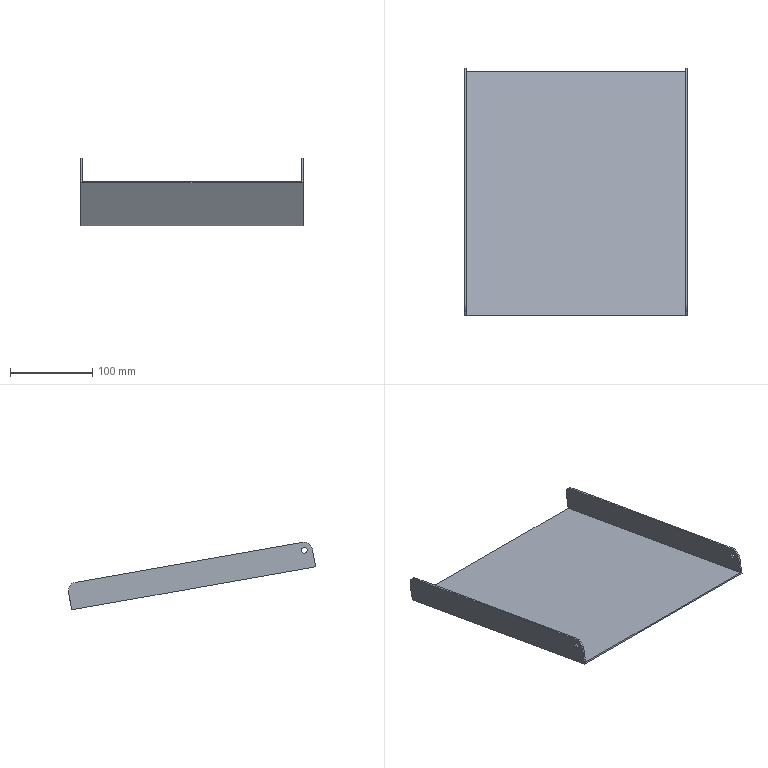Part | NX | features HB 2 | 1 solid | 16 faces | box 270 x 300.028 x 82.132 mm | volume 198086 mm3 | plane 10 | cylinder 6 | commonest cylinder face diameters 20 x4 7 x2
STEP:
#1=CARTESIAN_POINT('',(296.,686.06,-368.904));
#2=VERTEX_POINT('',#1);
#3=CARTESIAN_POINT('',(296.,686.966,-372.285));
#4=DIRECTION('',(1.,0.,0.));
#5=DIRECTION('',(0.,-0.2588,0.9659));
#6=AXIS2_PLACEMENT_3D('',#3,#4,#5);
#7=CIRCLE('',#6,3.5);
#8=EDGE_CURVE('',#2,#2,#7,.T.);
#9=ORIENTED_EDGE('',*,*,#8,.T.);
#10=EDGE_LOOP('',(#9));
#11=FACE_BOUND('',#10,.T.);
#12=CARTESIAN_POINT('',(294.,686.06,-368.904));
#13=VERTEX_POINT('',#12);
#14=CARTESIAN_POINT('',(294.,686.966,-372.285));
#15=DIRECTION('',(-1.,0.,0.));
#16=DIRECTION('',(0.,-0.2588,0.9659));
#17=AXIS2_PLACEMENT_3D('',#14,#15,#16);
#18=CIRCLE('',#17,3.5);
#19=EDGE_CURVE('',#13,#13,#18,.T.);
#20=ORIENTED_EDGE('',*,*,#19,.T.);
#21=EDGE_LOOP('',(#20));
#22=FACE_BOUND('',#21,.T.);
#23=CARTESIAN_POINT('',(-406.,686.966,-372.285));
#24=DIRECTION('',(1.,0.,0.));
#25=DIRECTION('',(0.,0.2588,-0.9659));
#26=AXIS2_PLACEMENT_3D('',#23,#24,#25);
#27=CYLINDRICAL_SURFACE('',#26,3.5);
#28=ADVANCED_FACE('',(#11,#22),#27,.F.);
#29=CARTESIAN_POINT('',(296.,965.062,-411.167));
#30=VERTEX_POINT('',#29);
#31=CARTESIAN_POINT('',(296.,688.702,-362.437));
#32=VERTEX_POINT('',#31);
#33=CARTESIAN_POINT('',(296.,564.245,-340.492));
#34=DIRECTION('',(0.,-0.9848,0.1736));
#35=VECTOR('',#34,1000.);
#36=LINE('',#33,#35);
#37=EDGE_CURVE('',#30,#32,#36,.T.);
#38=ORIENTED_EDGE('',*,*,#37,.F.);
#39=CARTESIAN_POINT('',(294.,965.062,-411.167));
#40=VERTEX_POINT('',#39);
#41=CARTESIAN_POINT('',(200.,965.062,-411.167));
#42=DIRECTION('',(1.,0.,0.));
#43=VECTOR('',#42,1000.);
#44=LINE('',#41,#43);
#45=EDGE_CURVE('',#40,#30,#44,.T.);
#46=ORIENTED_EDGE('',*,*,#45,.F.);
#47=CARTESIAN_POINT('',(294.,688.702,-362.437));
#48=VERTEX_POINT('',#47);
#49=CARTESIAN_POINT('',(294.,564.245,-340.492));
#50=DIRECTION('',(0.,-0.9848,0.1736));
#51=VECTOR('',#50,1000.);
#52=LINE('',#49,#51);
#53=EDGE_CURVE('',#40,#48,#52,.T.);
#54=ORIENTED_EDGE('',*,*,#53,.T.);
#55=CARTESIAN_POINT('',(200.,688.702,-362.437));
#56=DIRECTION('',(1.,0.,0.));
#57=VECTOR('',#56,1000.);
#58=LINE('',#55,#57);
#59=EDGE_CURVE('',#48,#32,#58,.T.);
#60=ORIENTED_EDGE('',*,*,#59,.T.);
#61=EDGE_LOOP('',(#38,#46,#54,#60));
#62=FACE_BOUND('',#61,.T.);
#63=CARTESIAN_POINT('',(200.,564.245,-340.492));
#64=DIRECTION('',(0.,-0.1736,-0.9848));
#65=DIRECTION('',(0.,0.9848,-0.1736));
#66=AXIS2_PLACEMENT_3D('',#63,#64,#65);
#67=PLANE('',#66);
#68=ADVANCED_FACE('',(#62),#67,.F.);
#69=CARTESIAN_POINT('',(296.,973.174,-422.751));
#70=VERTEX_POINT('',#69);
#71=CARTESIAN_POINT('',(296.,963.326,-421.015));
#72=DIRECTION('',(-1.,0.,0.));
#73=DIRECTION('',(0.,-0.2588,0.9659));
#74=AXIS2_PLACEMENT_3D('',#71,#72,#73);
#75=CIRCLE('',#74,10.);
#76=EDGE_CURVE('',#30,#70,#75,.T.);
#77=ORIENTED_EDGE('',*,*,#76,.T.);
#78=CARTESIAN_POINT('',(294.,973.174,-422.751));
#79=VERTEX_POINT('',#78);
#80=CARTESIAN_POINT('',(200.,973.174,-422.751));
#81=DIRECTION('',(-1.,0.,0.));
#82=VECTOR('',#81,1000.);
#83=LINE('',#80,#82);
#84=EDGE_CURVE('',#70,#79,#83,.T.);
#85=ORIENTED_EDGE('',*,*,#84,.T.);
#86=CARTESIAN_POINT('',(294.,963.326,-421.015));
#87=DIRECTION('',(1.,0.,0.));
#88=DIRECTION('',(0.,-0.2588,0.9659));
#89=AXIS2_PLACEMENT_3D('',#86,#87,#88);
#90=CIRCLE('',#89,10.);
#91=EDGE_CURVE('',#79,#40,#90,.T.);
#92=ORIENTED_EDGE('',*,*,#91,.T.);
#93=ORIENTED_EDGE('',*,*,#45,.T.);
#94=EDGE_LOOP('',(#77,#85,#92,#93));
#95=FACE_BOUND('',#94,.T.);
#96=CARTESIAN_POINT('',(200.,963.326,-421.015));
#97=DIRECTION('',(-1.,0.,0.));
#98=DIRECTION('',(0.,-0.2588,0.9659));
#99=AXIS2_PLACEMENT_3D('',#96,#97,#98);
#100=CYLINDRICAL_SURFACE('',#99,10.);
#101=ADVANCED_FACE('',(#95),#100,.T.);
#102=ORIENTED_EDGE('',*,*,#53,.F.);
#103=ORIENTED_EDGE('',*,*,#91,.F.);
#104=CARTESIAN_POINT('',(294.,969.354,-444.417));
#105=VERTEX_POINT('',#104);
#106=CARTESIAN_POINT('',(294.,969.701,-442.448));
#107=DIRECTION('',(0.,0.1736,0.9848));
#108=VECTOR('',#107,1000.);
#109=LINE('',#106,#108);
#110=EDGE_CURVE('',#105,#79,#109,.T.);
#111=ORIENTED_EDGE('',*,*,#110,.F.);
#112=CARTESIAN_POINT('',(294.,673.298,-392.215));
#113=VERTEX_POINT('',#112);
#114=CARTESIAN_POINT('',(294.,558.689,-372.006));
#115=DIRECTION('',(0.,0.9848,-0.1736));
#116=VECTOR('',#115,1000.);
#117=LINE('',#114,#116);
#118=EDGE_CURVE('',#113,#105,#117,.T.);
#119=ORIENTED_EDGE('',*,*,#118,.F.);
#120=CARTESIAN_POINT('',(294.,677.118,-370.549));
#121=VERTEX_POINT('',#120);
#122=CARTESIAN_POINT('',(294.,673.645,-390.245));
#123=DIRECTION('',(0.,0.1736,0.9848));
#124=VECTOR('',#123,1000.);
#125=LINE('',#122,#124);
#126=EDGE_CURVE('',#113,#121,#125,.T.);
#127=ORIENTED_EDGE('',*,*,#126,.T.);
#128=CARTESIAN_POINT('',(294.,686.966,-372.285));
#129=DIRECTION('',(-1.,0.,0.));
#130=DIRECTION('',(0.,0.5736,0.8192));
#131=AXIS2_PLACEMENT_3D('',#128,#129,#130);
#132=CIRCLE('',#131,10.);
#133=EDGE_CURVE('',#121,#48,#132,.T.);
#134=ORIENTED_EDGE('',*,*,#133,.T.);
#135=EDGE_LOOP('',(#102,#103,#111,#119,#127,#134));
#136=FACE_BOUND('',#135,.T.);
#137=ORIENTED_EDGE('',*,*,#19,.F.);
#138=EDGE_LOOP('',(#137));
#139=FACE_BOUND('',#138,.T.);
#140=CARTESIAN_POINT('',(294.,559.036,-370.036));
#141=DIRECTION('',(1.,0.,0.));
#142=DIRECTION('',(0.,0.2588,-0.9659));
#143=AXIS2_PLACEMENT_3D('',#140,#141,#142);
#144=PLANE('',#143);
#145=ADVANCED_FACE('',(#136,#139),#144,.F.);
#146=CARTESIAN_POINT('',(296.,677.118,-370.549));
#147=VERTEX_POINT('',#146);
#148=CARTESIAN_POINT('',(296.,686.966,-372.285));
#149=DIRECTION('',(1.,0.,0.));
#150=DIRECTION('',(0.,0.5736,0.8192));
#151=AXIS2_PLACEMENT_3D('',#148,#149,#150);
#152=CIRCLE('',#151,10.);
#153=EDGE_CURVE('',#32,#147,#152,.T.);
#154=ORIENTED_EDGE('',*,*,#153,.F.);
#155=ORIENTED_EDGE('',*,*,#59,.F.);
#156=ORIENTED_EDGE('',*,*,#133,.F.);
#157=CARTESIAN_POINT('',(260.,677.118,-370.549));
#158=DIRECTION('',(-1.,0.,0.));
#159=VECTOR('',#158,1000.);
#160=LINE('',#157,#159);
#161=EDGE_CURVE('',#147,#121,#160,.T.);
#162=ORIENTED_EDGE('',*,*,#161,.F.);
#163=EDGE_LOOP('',(#154,#155,#156,#162));
#164=FACE_BOUND('',#163,.T.);
#165=CARTESIAN_POINT('',(200.,686.966,-372.285));
#166=DIRECTION('',(-1.,0.,0.));
#167=DIRECTION('',(0.,0.5736,0.8192));
#168=AXIS2_PLACEMENT_3D('',#165,#166,#167);
#169=CYLINDRICAL_SURFACE('',#168,10.);
#170=ADVANCED_FACE('',(#164),#169,.T.);
#171=ORIENTED_EDGE('',*,*,#76,.F.);
#172=ORIENTED_EDGE('',*,*,#37,.T.);
#173=ORIENTED_EDGE('',*,*,#153,.T.);
#174=CARTESIAN_POINT('',(296.,673.645,-390.245));
#175=VERTEX_POINT('',#174);
#176=CARTESIAN_POINT('',(296.,673.645,-390.245));
#177=DIRECTION('',(0.,0.1736,0.9848));
#178=VECTOR('',#177,1000.);
#179=LINE('',#176,#178);
#180=EDGE_CURVE('',#175,#147,#179,.T.);
#181=ORIENTED_EDGE('',*,*,#180,.F.);
#182=CARTESIAN_POINT('',(296.,969.701,-442.448));
#183=VERTEX_POINT('',#182);
#184=CARTESIAN_POINT('',(296.,559.036,-370.036));
#185=DIRECTION('',(0.,-0.9848,0.1736));
#186=VECTOR('',#185,1000.);
#187=LINE('',#184,#186);
#188=EDGE_CURVE('',#183,#175,#187,.T.);
#189=ORIENTED_EDGE('',*,*,#188,.F.);
#190=CARTESIAN_POINT('',(296.,969.701,-442.448));
#191=DIRECTION('',(0.,0.1736,0.9848));
#192=VECTOR('',#191,1000.);
#193=LINE('',#190,#192);
#194=EDGE_CURVE('',#183,#70,#193,.T.);
#195=ORIENTED_EDGE('',*,*,#194,.T.);
#196=EDGE_LOOP('',(#171,#172,#173,#181,#189,#195));
#197=FACE_BOUND('',#196,.T.);
#198=ORIENTED_EDGE('',*,*,#8,.F.);
#199=EDGE_LOOP('',(#198));
#200=FACE_BOUND('',#199,.T.);
#201=CARTESIAN_POINT('',(296.,559.036,-370.036));
#202=DIRECTION('',(1.,0.,0.));
#203=DIRECTION('',(0.,-0.2588,0.9659));
#204=AXIS2_PLACEMENT_3D('',#201,#202,#203);
#205=PLANE('',#204);
#206=ADVANCED_FACE('',(#197,#200),#205,.T.);
#207=CARTESIAN_POINT('',(562.,673.645,-390.245));
#208=VERTEX_POINT('',#207);
#209=CARTESIAN_POINT('',(260.,673.645,-390.245));
#210=DIRECTION('',(1.,0.,0.));
#211=VECTOR('',#210,1000.);
#212=LINE('',#209,#211);
#213=EDGE_CURVE('',#175,#208,#212,.T.);
#214=ORIENTED_EDGE('',*,*,#213,.F.);
#215=ORIENTED_EDGE('',*,*,#180,.T.);
#216=ORIENTED_EDGE('',*,*,#161,.T.);
#217=ORIENTED_EDGE('',*,*,#126,.F.);
#218=CARTESIAN_POINT('',(564.,673.298,-392.215));
#219=VERTEX_POINT('',#218);
#220=CARTESIAN_POINT('',(260.,673.298,-392.215));
#221=DIRECTION('',(1.,0.,0.));
#222=VECTOR('',#221,1000.);
#223=LINE('',#220,#222);
#224=EDGE_CURVE('',#113,#219,#223,.T.);
#225=ORIENTED_EDGE('',*,*,#224,.T.);
#226=CARTESIAN_POINT('',(564.,677.118,-370.549));
#227=VERTEX_POINT('',#226);
#228=CARTESIAN_POINT('',(564.,673.645,-390.245));
#229=DIRECTION('',(0.,0.1736,0.9848));
#230=VECTOR('',#229,1000.);
#231=LINE('',#228,#230);
#232=EDGE_CURVE('',#219,#227,#231,.T.);
#233=ORIENTED_EDGE('',*,*,#232,.T.);
#234=CARTESIAN_POINT('',(562.,677.118,-370.549));
#235=VERTEX_POINT('',#234);
#236=CARTESIAN_POINT('',(260.,677.118,-370.549));
#237=DIRECTION('',(-1.,0.,0.));
#238=VECTOR('',#237,1000.);
#239=LINE('',#236,#238);
#240=EDGE_CURVE('',#227,#235,#239,.T.);
#241=ORIENTED_EDGE('',*,*,#240,.T.);
#242=CARTESIAN_POINT('',(562.,673.645,-390.245));
#243=DIRECTION('',(0.,0.1736,0.9848));
#244=VECTOR('',#243,1000.);
#245=LINE('',#242,#244);
#246=EDGE_CURVE('',#208,#235,#245,.T.);
#247=ORIENTED_EDGE('',*,*,#246,.F.);
#248=EDGE_LOOP('',(#214,#215,#216,#217,#225,#233,#241,#247));
#249=FACE_BOUND('',#248,.T.);
#250=CARTESIAN_POINT('',(260.,673.645,-390.245));
#251=DIRECTION('',(0.,0.9848,-0.1736));
#252=DIRECTION('',(0.,-0.1736,-0.9848));
#253=AXIS2_PLACEMENT_3D('',#250,#251,#252);
#254=PLANE('',#253);
#255=ADVANCED_FACE('',(#249),#254,.F.);
#256=ORIENTED_EDGE('',*,*,#194,.F.);
#257=CARTESIAN_POINT('',(562.,969.701,-442.448));
#258=VERTEX_POINT('',#257);
#259=CARTESIAN_POINT('',(260.,969.701,-442.448));
#260=DIRECTION('',(1.,0.,0.));
#261=VECTOR('',#260,1000.);
#262=LINE('',#259,#261);
#263=EDGE_CURVE('',#183,#258,#262,.T.);
#264=ORIENTED_EDGE('',*,*,#263,.T.);
#265=CARTESIAN_POINT('',(562.,973.174,-422.751));
#266=VERTEX_POINT('',#265);
#267=CARTESIAN_POINT('',(562.,969.701,-442.448));
#268=DIRECTION('',(0.,0.1736,0.9848));
#269=VECTOR('',#268,1000.);
#270=LINE('',#267,#269);
#271=EDGE_CURVE('',#258,#266,#270,.T.);
#272=ORIENTED_EDGE('',*,*,#271,.T.);
#273=CARTESIAN_POINT('',(564.,973.174,-422.751));
#274=VERTEX_POINT('',#273);
#275=CARTESIAN_POINT('',(259.,973.174,-422.751));
#276=DIRECTION('',(-1.,0.,0.));
#277=VECTOR('',#276,1000.);
#278=LINE('',#275,#277);
#279=EDGE_CURVE('',#274,#266,#278,.T.);
#280=ORIENTED_EDGE('',*,*,#279,.F.);
#281=CARTESIAN_POINT('',(564.,969.354,-444.417));
#282=VERTEX_POINT('',#281);
#283=CARTESIAN_POINT('',(564.,969.701,-442.448));
#284=DIRECTION('',(0.,0.1736,0.9848));
#285=VECTOR('',#284,1000.);
#286=LINE('',#283,#285);
#287=EDGE_CURVE('',#282,#274,#286,.T.);
#288=ORIENTED_EDGE('',*,*,#287,.F.);
#289=CARTESIAN_POINT('',(260.,969.354,-444.417));
#290=DIRECTION('',(1.,0.,0.));
#291=VECTOR('',#290,1000.);
#292=LINE('',#289,#291);
#293=EDGE_CURVE('',#105,#282,#292,.T.);
#294=ORIENTED_EDGE('',*,*,#293,.F.);
#295=ORIENTED_EDGE('',*,*,#110,.T.);
#296=ORIENTED_EDGE('',*,*,#84,.F.);
#297=EDGE_LOOP('',(#256,#264,#272,#280,#288,#294,#295,#296));
#298=FACE_BOUND('',#297,.T.);
#299=CARTESIAN_POINT('',(260.,969.701,-442.448));
#300=DIRECTION('',(0.,-0.9848,0.1736));
#301=DIRECTION('',(0.,-0.1736,-0.9848));
#302=AXIS2_PLACEMENT_3D('',#299,#300,#301);
#303=PLANE('',#302);
#304=ADVANCED_FACE('',(#298),#303,.F.);
#305=ORIENTED_EDGE('',*,*,#118,.T.);
#306=ORIENTED_EDGE('',*,*,#293,.T.);
#307=CARTESIAN_POINT('',(564.,558.689,-372.006));
#308=DIRECTION('',(0.,-0.9848,0.1736));
#309=VECTOR('',#308,1000.);
#310=LINE('',#307,#309);
#311=EDGE_CURVE('',#282,#219,#310,.T.);
#312=ORIENTED_EDGE('',*,*,#311,.T.);
#313=ORIENTED_EDGE('',*,*,#224,.F.);
#314=EDGE_LOOP('',(#305,#306,#312,#313));
#315=FACE_BOUND('',#314,.T.);
#316=CARTESIAN_POINT('',(260.,558.689,-372.006));
#317=DIRECTION('',(0.,0.1736,0.9848));
#318=DIRECTION('',(1.,0.,0.));
#319=AXIS2_PLACEMENT_3D('',#316,#317,#318);
#320=PLANE('',#319);
#321=ADVANCED_FACE('',(#315),#320,.F.);
#322=ORIENTED_EDGE('',*,*,#263,.F.);
#323=ORIENTED_EDGE('',*,*,#188,.T.);
#324=ORIENTED_EDGE('',*,*,#213,.T.);
#325=CARTESIAN_POINT('',(562.,559.036,-370.036));
#326=DIRECTION('',(0.,0.9848,-0.1736));
#327=VECTOR('',#326,1000.);
#328=LINE('',#325,#327);
#329=EDGE_CURVE('',#208,#258,#328,.T.);
#330=ORIENTED_EDGE('',*,*,#329,.T.);
#331=EDGE_LOOP('',(#322,#323,#324,#330));
#332=FACE_BOUND('',#331,.T.);
#333=CARTESIAN_POINT('',(260.,559.036,-370.036));
#334=DIRECTION('',(0.,0.1736,0.9848));
#335=DIRECTION('',(1.,0.,0.));
#336=AXIS2_PLACEMENT_3D('',#333,#334,#335);
#337=PLANE('',#336);
#338=ADVANCED_FACE('',(#332),#337,.T.);
#339=CARTESIAN_POINT('',(564.,687.872,-375.666));
#340=VERTEX_POINT('',#339);
#341=CARTESIAN_POINT('',(564.,686.966,-372.285));
#342=DIRECTION('',(1.,0.,0.));
#343=DIRECTION('',(0.,0.2588,-0.9659));
#344=AXIS2_PLACEMENT_3D('',#341,#342,#343);
#345=CIRCLE('',#344,3.5);
#346=EDGE_CURVE('',#340,#340,#345,.T.);
#347=ORIENTED_EDGE('',*,*,#346,.F.);
#348=EDGE_LOOP('',(#347));
#349=FACE_BOUND('',#348,.T.);
#350=ORIENTED_EDGE('',*,*,#311,.F.);
#351=ORIENTED_EDGE('',*,*,#287,.T.);
#352=CARTESIAN_POINT('',(564.,965.062,-411.167));
#353=VERTEX_POINT('',#352);
#354=CARTESIAN_POINT('',(564.,963.326,-421.015));
#355=DIRECTION('',(-1.,0.,0.));
#356=DIRECTION('',(0.,0.2588,-0.9659));
#357=AXIS2_PLACEMENT_3D('',#354,#355,#356);
#358=CIRCLE('',#357,10.);
#359=EDGE_CURVE('',#353,#274,#358,.T.);
#360=ORIENTED_EDGE('',*,*,#359,.F.);
#361=CARTESIAN_POINT('',(564.,688.702,-362.437));
#362=VERTEX_POINT('',#361);
#363=CARTESIAN_POINT('',(564.,564.245,-340.492));
#364=DIRECTION('',(0.,-0.9848,0.1736));
#365=VECTOR('',#364,1000.);
#366=LINE('',#363,#365);
#367=EDGE_CURVE('',#353,#362,#366,.T.);
#368=ORIENTED_EDGE('',*,*,#367,.T.);
#369=CARTESIAN_POINT('',(564.,686.966,-372.285));
#370=DIRECTION('',(1.,0.,0.));
#371=DIRECTION('',(0.,-0.5736,-0.8192));
#372=AXIS2_PLACEMENT_3D('',#369,#370,#371);
#373=CIRCLE('',#372,10.);
#374=EDGE_CURVE('',#362,#227,#373,.T.);
#375=ORIENTED_EDGE('',*,*,#374,.T.);
#376=ORIENTED_EDGE('',*,*,#232,.F.);
#377=EDGE_LOOP('',(#350,#351,#360,#368,#375,#376));
#378=FACE_BOUND('',#377,.T.);
#379=CARTESIAN_POINT('',(564.,559.036,-370.036));
#380=DIRECTION('',(-1.,0.,0.));
#381=DIRECTION('',(0.,-0.2588,0.9659));
#382=AXIS2_PLACEMENT_3D('',#379,#380,#381);
#383=PLANE('',#382);
#384=ADVANCED_FACE('',(#349,#378),#383,.F.);
#385=ORIENTED_EDGE('',*,*,#367,.F.);
#386=CARTESIAN_POINT('',(562.,965.062,-411.167));
#387=VERTEX_POINT('',#386);
#388=CARTESIAN_POINT('',(517.,965.062,-411.167));
#389=DIRECTION('',(1.,0.,0.));
#390=VECTOR('',#389,1000.);
#391=LINE('',#388,#390);
#392=EDGE_CURVE('',#387,#353,#391,.T.);
#393=ORIENTED_EDGE('',*,*,#392,.F.);
#394=CARTESIAN_POINT('',(562.,688.702,-362.437));
#395=VERTEX_POINT('',#394);
#396=CARTESIAN_POINT('',(562.,564.245,-340.492));
#397=DIRECTION('',(0.,-0.9848,0.1736));
#398=VECTOR('',#397,1000.);
#399=LINE('',#396,#398);
#400=EDGE_CURVE('',#387,#395,#399,.T.);
#401=ORIENTED_EDGE('',*,*,#400,.T.);
#402=CARTESIAN_POINT('',(517.,688.702,-362.437));
#403=DIRECTION('',(1.,0.,0.));
#404=VECTOR('',#403,1000.);
#405=LINE('',#402,#404);
#406=EDGE_CURVE('',#395,#362,#405,.T.);
#407=ORIENTED_EDGE('',*,*,#406,.T.);
#408=EDGE_LOOP('',(#385,#393,#401,#407));
#409=FACE_BOUND('',#408,.T.);
#410=CARTESIAN_POINT('',(517.,564.245,-340.492));
#411=DIRECTION('',(0.,-0.1736,-0.9848));
#412=DIRECTION('',(0.,0.9848,-0.1736));
#413=AXIS2_PLACEMENT_3D('',#410,#411,#412);
#414=PLANE('',#413);
#415=ADVANCED_FACE('',(#409),#414,.F.);
#416=CARTESIAN_POINT('',(562.,687.872,-375.666));
#417=VERTEX_POINT('',#416);
#418=CARTESIAN_POINT('',(562.,686.966,-372.285));
#419=DIRECTION('',(1.,0.,0.));
#420=DIRECTION('',(0.,0.2588,-0.9659));
#421=AXIS2_PLACEMENT_3D('',#418,#419,#420);
#422=CIRCLE('',#421,3.5);
#423=EDGE_CURVE('',#417,#417,#422,.T.);
#424=ORIENTED_EDGE('',*,*,#423,.T.);
#425=EDGE_LOOP('',(#424));
#426=FACE_BOUND('',#425,.T.);
#427=ORIENTED_EDGE('',*,*,#329,.F.);
#428=ORIENTED_EDGE('',*,*,#246,.T.);
#429=CARTESIAN_POINT('',(562.,686.966,-372.285));
#430=DIRECTION('',(-1.,0.,0.));
#431=DIRECTION('',(0.,-0.5736,-0.8192));
#432=AXIS2_PLACEMENT_3D('',#429,#430,#431);
#433=CIRCLE('',#432,10.);
#434=EDGE_CURVE('',#235,#395,#433,.T.);
#435=ORIENTED_EDGE('',*,*,#434,.T.);
#436=ORIENTED_EDGE('',*,*,#400,.F.);
#437=CARTESIAN_POINT('',(562.,963.326,-421.015));
#438=DIRECTION('',(1.,0.,0.));
#439=DIRECTION('',(0.,0.2588,-0.9659));
#440=AXIS2_PLACEMENT_3D('',#437,#438,#439);
#441=CIRCLE('',#440,10.);
#442=EDGE_CURVE('',#266,#387,#441,.T.);
#443=ORIENTED_EDGE('',*,*,#442,.F.);
#444=ORIENTED_EDGE('',*,*,#271,.F.);
#445=EDGE_LOOP('',(#427,#428,#435,#436,#443,#444));
#446=FACE_BOUND('',#445,.T.);
#447=CARTESIAN_POINT('',(562.,559.036,-370.036));
#448=DIRECTION('',(-1.,0.,0.));
#449=DIRECTION('',(0.,-0.2588,0.9659));
#450=AXIS2_PLACEMENT_3D('',#447,#448,#449);
#451=PLANE('',#450);
#452=ADVANCED_FACE('',(#426,#446),#451,.T.);
#453=ORIENTED_EDGE('',*,*,#442,.T.);
#454=ORIENTED_EDGE('',*,*,#392,.T.);
#455=ORIENTED_EDGE('',*,*,#359,.T.);
#456=ORIENTED_EDGE('',*,*,#279,.T.);
#457=EDGE_LOOP('',(#453,#454,#455,#456));
#458=FACE_BOUND('',#457,.T.);
#459=CARTESIAN_POINT('',(259.,963.326,-421.015));
#460=DIRECTION('',(1.,0.,0.));
#461=DIRECTION('',(0.,0.2588,-0.9659));
#462=AXIS2_PLACEMENT_3D('',#459,#460,#461);
#463=CYLINDRICAL_SURFACE('',#462,10.);
#464=ADVANCED_FACE('',(#458),#463,.T.);
#465=ORIENTED_EDGE('',*,*,#434,.F.);
#466=ORIENTED_EDGE('',*,*,#240,.F.);
#467=ORIENTED_EDGE('',*,*,#374,.F.);
#468=ORIENTED_EDGE('',*,*,#406,.F.);
#469=EDGE_LOOP('',(#465,#466,#467,#468));
#470=FACE_BOUND('',#469,.T.);
#471=CARTESIAN_POINT('',(259.,686.966,-372.285));
#472=DIRECTION('',(1.,0.,0.));
#473=DIRECTION('',(0.,-0.5736,-0.8192));
#474=AXIS2_PLACEMENT_3D('',#471,#472,#473);
#475=CYLINDRICAL_SURFACE('',#474,10.);
#476=ADVANCED_FACE('',(#470),#475,.T.);
#477=ORIENTED_EDGE('',*,*,#423,.F.);
#478=EDGE_LOOP('',(#477));
#479=FACE_BOUND('',#478,.T.);
#480=ORIENTED_EDGE('',*,*,#346,.T.);
#481=EDGE_LOOP('',(#480));
#482=FACE_BOUND('',#481,.T.);
#483=CARTESIAN_POINT('',(519.,686.966,-372.285));
#484=DIRECTION('',(-1.,0.,0.));
#485=DIRECTION('',(0.,-0.2588,0.9659));
#486=AXIS2_PLACEMENT_3D('',#483,#484,#485);
#487=CYLINDRICAL_SURFACE('',#486,3.5);
#488=ADVANCED_FACE('',(#479,#482),#487,.F.);
#489=CLOSED_SHELL('',(#28,#68,#101,#145,#170,#206,#255,#304,#321,#338,#384,#415,#452,#464,#476,#488));
#490=MANIFOLD_SOLID_BREP('',#489);
#491=(LENGTH_UNIT()NAMED_UNIT(*)SI_UNIT(.MILLI.,.METRE.));
#492=UNCERTAINTY_MEASURE_WITH_UNIT(LENGTH_MEASURE(0.00001),#491,'','');
#493=(NAMED_UNIT(*)PLANE_ANGLE_UNIT()SI_UNIT($,.RADIAN.));
#494=(NAMED_UNIT(*)SI_UNIT($,.STERADIAN.)SOLID_ANGLE_UNIT());
#495=(GEOMETRIC_REPRESENTATION_CONTEXT(3)GLOBAL_UNCERTAINTY_ASSIGNED_CONTEXT((#492))GLOBAL_UNIT_ASSIGNED_CONTEXT((#491,#493,#494))REPRESENTATION_CONTEXT('',''));
#496=ADVANCED_BREP_SHAPE_REPRESENTATION('',(#490),#495);